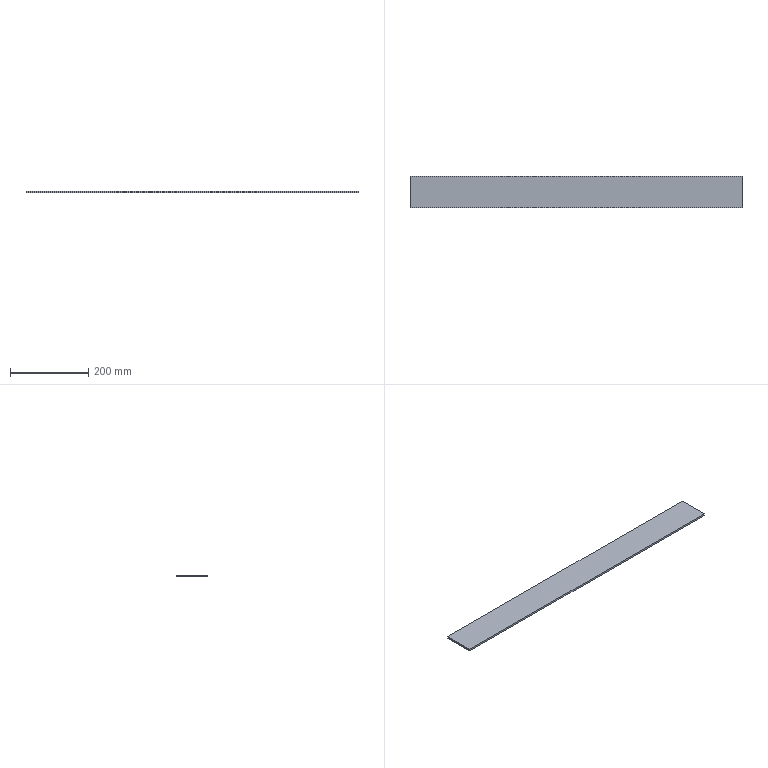Part | NX | features BREP 1 | 1 solid | 6 faces | box 850 x 80 x 5 mm | volume 340000 mm3 | plane 6
STEP:
#1=CARTESIAN_POINT('',(425.,-40.,0.));
#2=VERTEX_POINT('',#1);
#3=CARTESIAN_POINT('',(425.,40.,0.));
#4=VERTEX_POINT('',#3);
#5=CARTESIAN_POINT('',(425.,-40.,0.));
#6=DIRECTION('',(0.,1.,0.));
#7=VECTOR('',#6,1000.);
#8=LINE('',#5,#7);
#9=EDGE_CURVE('',#2,#4,#8,.T.);
#10=ORIENTED_EDGE('',*,*,#9,.F.);
#11=CARTESIAN_POINT('',(425.,-40.,-5.));
#12=VERTEX_POINT('',#11);
#13=CARTESIAN_POINT('',(425.,-40.,-5.));
#14=DIRECTION('',(0.,0.,1.));
#15=VECTOR('',#14,1000.);
#16=LINE('',#13,#15);
#17=EDGE_CURVE('',#12,#2,#16,.T.);
#18=ORIENTED_EDGE('',*,*,#17,.F.);
#19=CARTESIAN_POINT('',(425.,40.,-5.));
#20=VERTEX_POINT('',#19);
#21=CARTESIAN_POINT('',(425.,-40.,-5.));
#22=DIRECTION('',(0.,1.,0.));
#23=VECTOR('',#22,1000.);
#24=LINE('',#21,#23);
#25=EDGE_CURVE('',#12,#20,#24,.T.);
#26=ORIENTED_EDGE('',*,*,#25,.T.);
#27=CARTESIAN_POINT('',(425.,40.,-5.));
#28=DIRECTION('',(0.,0.,1.));
#29=VECTOR('',#28,1000.);
#30=LINE('',#27,#29);
#31=EDGE_CURVE('',#20,#4,#30,.T.);
#32=ORIENTED_EDGE('',*,*,#31,.T.);
#33=EDGE_LOOP('',(#10,#18,#26,#32));
#34=FACE_BOUND('',#33,.T.);
#35=CARTESIAN_POINT('',(425.,-40.,-5.));
#36=DIRECTION('',(1.,0.,0.));
#37=DIRECTION('',(0.,0.,-1.));
#38=AXIS2_PLACEMENT_3D('',#35,#36,#37);
#39=PLANE('',#38);
#40=ADVANCED_FACE('',(#34),#39,.T.);
#41=CARTESIAN_POINT('',(-425.,-40.,0.));
#42=VERTEX_POINT('',#41);
#43=CARTESIAN_POINT('',(-425.,-40.,0.));
#44=DIRECTION('',(1.,0.,0.));
#45=VECTOR('',#44,1000.);
#46=LINE('',#43,#45);
#47=EDGE_CURVE('',#42,#2,#46,.T.);
#48=ORIENTED_EDGE('',*,*,#47,.F.);
#49=CARTESIAN_POINT('',(-425.,-40.,-5.));
#50=VERTEX_POINT('',#49);
#51=CARTESIAN_POINT('',(-425.,-40.,-5.));
#52=DIRECTION('',(0.,0.,1.));
#53=VECTOR('',#52,1000.);
#54=LINE('',#51,#53);
#55=EDGE_CURVE('',#50,#42,#54,.T.);
#56=ORIENTED_EDGE('',*,*,#55,.F.);
#57=CARTESIAN_POINT('',(-425.,-40.,-5.));
#58=DIRECTION('',(1.,0.,0.));
#59=VECTOR('',#58,1000.);
#60=LINE('',#57,#59);
#61=EDGE_CURVE('',#50,#12,#60,.T.);
#62=ORIENTED_EDGE('',*,*,#61,.T.);
#63=ORIENTED_EDGE('',*,*,#17,.T.);
#64=EDGE_LOOP('',(#48,#56,#62,#63));
#65=FACE_BOUND('',#64,.T.);
#66=CARTESIAN_POINT('',(-425.,-40.,-5.));
#67=DIRECTION('',(0.,-1.,0.));
#68=DIRECTION('',(0.,0.,-1.));
#69=AXIS2_PLACEMENT_3D('',#66,#67,#68);
#70=PLANE('',#69);
#71=ADVANCED_FACE('',(#65),#70,.T.);
#72=CARTESIAN_POINT('',(-425.,40.,0.));
#73=VERTEX_POINT('',#72);
#74=CARTESIAN_POINT('',(-425.,-40.,0.));
#75=DIRECTION('',(0.,-1.,0.));
#76=VECTOR('',#75,1000.);
#77=LINE('',#74,#76);
#78=EDGE_CURVE('',#73,#42,#77,.T.);
#79=ORIENTED_EDGE('',*,*,#78,.F.);
#80=CARTESIAN_POINT('',(-425.,40.,-5.));
#81=VERTEX_POINT('',#80);
#82=CARTESIAN_POINT('',(-425.,40.,-5.));
#83=DIRECTION('',(0.,0.,1.));
#84=VECTOR('',#83,1000.);
#85=LINE('',#82,#84);
#86=EDGE_CURVE('',#81,#73,#85,.T.);
#87=ORIENTED_EDGE('',*,*,#86,.F.);
#88=CARTESIAN_POINT('',(-425.,-40.,-5.));
#89=DIRECTION('',(0.,-1.,0.));
#90=VECTOR('',#89,1000.);
#91=LINE('',#88,#90);
#92=EDGE_CURVE('',#81,#50,#91,.T.);
#93=ORIENTED_EDGE('',*,*,#92,.T.);
#94=ORIENTED_EDGE('',*,*,#55,.T.);
#95=EDGE_LOOP('',(#79,#87,#93,#94));
#96=FACE_BOUND('',#95,.T.);
#97=CARTESIAN_POINT('',(-425.,-40.,-5.));
#98=DIRECTION('',(-1.,0.,0.));
#99=DIRECTION('',(0.,0.,1.));
#100=AXIS2_PLACEMENT_3D('',#97,#98,#99);
#101=PLANE('',#100);
#102=ADVANCED_FACE('',(#96),#101,.T.);
#103=CARTESIAN_POINT('',(-425.,40.,0.));
#104=DIRECTION('',(-1.,0.,0.));
#105=VECTOR('',#104,1000.);
#106=LINE('',#103,#105);
#107=EDGE_CURVE('',#4,#73,#106,.T.);
#108=ORIENTED_EDGE('',*,*,#107,.F.);
#109=ORIENTED_EDGE('',*,*,#31,.F.);
#110=CARTESIAN_POINT('',(-425.,40.,-5.));
#111=DIRECTION('',(-1.,0.,0.));
#112=VECTOR('',#111,1000.);
#113=LINE('',#110,#112);
#114=EDGE_CURVE('',#20,#81,#113,.T.);
#115=ORIENTED_EDGE('',*,*,#114,.T.);
#116=ORIENTED_EDGE('',*,*,#86,.T.);
#117=EDGE_LOOP('',(#108,#109,#115,#116));
#118=FACE_BOUND('',#117,.T.);
#119=CARTESIAN_POINT('',(-425.,40.,-5.));
#120=DIRECTION('',(0.,1.,0.));
#121=DIRECTION('',(0.,0.,1.));
#122=AXIS2_PLACEMENT_3D('',#119,#120,#121);
#123=PLANE('',#122);
#124=ADVANCED_FACE('',(#118),#123,.T.);
#125=ORIENTED_EDGE('',*,*,#25,.F.);
#126=ORIENTED_EDGE('',*,*,#61,.F.);
#127=ORIENTED_EDGE('',*,*,#92,.F.);
#128=ORIENTED_EDGE('',*,*,#114,.F.);
#129=EDGE_LOOP('',(#125,#126,#127,#128));
#130=FACE_BOUND('',#129,.T.);
#131=CARTESIAN_POINT('',(0.,0.,-5.));
#132=DIRECTION('',(0.,0.,-1.));
#133=DIRECTION('',(-1.,0.,0.));
#134=AXIS2_PLACEMENT_3D('',#131,#132,#133);
#135=PLANE('',#134);
#136=ADVANCED_FACE('',(#130),#135,.T.);
#137=ORIENTED_EDGE('',*,*,#9,.T.);
#138=ORIENTED_EDGE('',*,*,#107,.T.);
#139=ORIENTED_EDGE('',*,*,#78,.T.);
#140=ORIENTED_EDGE('',*,*,#47,.T.);
#141=EDGE_LOOP('',(#137,#138,#139,#140));
#142=FACE_BOUND('',#141,.T.);
#143=CARTESIAN_POINT('',(0.,0.,0.));
#144=DIRECTION('',(0.,0.,-1.));
#145=DIRECTION('',(-1.,0.,0.));
#146=AXIS2_PLACEMENT_3D('',#143,#144,#145);
#147=PLANE('',#146);
#148=ADVANCED_FACE('',(#142),#147,.F.);
#149=CLOSED_SHELL('',(#40,#71,#102,#124,#136,#148));
#150=MANIFOLD_SOLID_BREP('',#149);
#151=(LENGTH_UNIT()NAMED_UNIT(*)SI_UNIT(.MILLI.,.METRE.));
#152=UNCERTAINTY_MEASURE_WITH_UNIT(LENGTH_MEASURE(0.00001),#151,'','');
#153=(NAMED_UNIT(*)PLANE_ANGLE_UNIT()SI_UNIT($,.RADIAN.));
#154=(NAMED_UNIT(*)SI_UNIT($,.STERADIAN.)SOLID_ANGLE_UNIT());
#155=(GEOMETRIC_REPRESENTATION_CONTEXT(3)GLOBAL_UNCERTAINTY_ASSIGNED_CONTEXT((#152))GLOBAL_UNIT_ASSIGNED_CONTEXT((#151,#153,#154))REPRESENTATION_CONTEXT('',''));
#156=ADVANCED_BREP_SHAPE_REPRESENTATION('',(#150),#155);